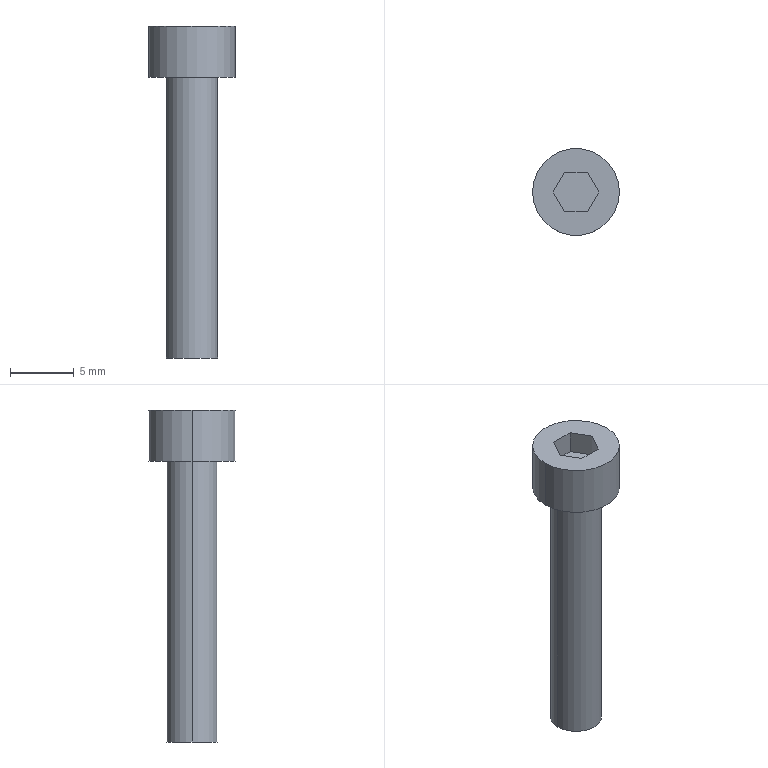Part | SolidWorks | features BaseBody 1 | 1 solid | 14 faces | box 6.8 x 6.8 x 26 mm | volume 406.575 mm3 | plane 10 | cylinder 4 | commonest cylinder face diameters 4 x2 6.8 x2
STEP:
#1=CARTESIAN_POINT('',(2.,0.,-22.));
#2=VERTEX_POINT('',#1);
#3=CARTESIAN_POINT('',(-2.,0.,-22.));
#4=VERTEX_POINT('',#3);
#5=CARTESIAN_POINT('',(0.,0.,-22.));
#6=DIRECTION('',(0.,0.,1.));
#7=DIRECTION('',(1.,0.,0.));
#8=AXIS2_PLACEMENT_3D('',#5,#6,#7);
#9=CIRCLE('',#8,2.);
#10=EDGE_CURVE('',#2,#4,#9,.T.);
#11=ORIENTED_EDGE('',*,*,#10,.T.);
#12=CARTESIAN_POINT('',(-2.,0.,0.));
#13=VERTEX_POINT('',#12);
#14=CARTESIAN_POINT('',(-2.,0.,-22.));
#15=DIRECTION('',(0.,0.,1.));
#16=VECTOR('',#15,1000.);
#17=LINE('',#14,#16);
#18=EDGE_CURVE('',#4,#13,#17,.T.);
#19=ORIENTED_EDGE('',*,*,#18,.T.);
#20=CARTESIAN_POINT('',(2.,0.,0.));
#21=VERTEX_POINT('',#20);
#22=CARTESIAN_POINT('',(0.,0.,0.));
#23=DIRECTION('',(0.,0.,-1.));
#24=DIRECTION('',(1.,0.,0.));
#25=AXIS2_PLACEMENT_3D('',#22,#23,#24);
#26=CIRCLE('',#25,2.);
#27=EDGE_CURVE('',#13,#21,#26,.T.);
#28=ORIENTED_EDGE('',*,*,#27,.T.);
#29=CARTESIAN_POINT('',(2.,0.,-22.));
#30=DIRECTION('',(0.,0.,1.));
#31=VECTOR('',#30,1000.);
#32=LINE('',#29,#31);
#33=EDGE_CURVE('',#2,#21,#32,.T.);
#34=ORIENTED_EDGE('',*,*,#33,.F.);
#35=EDGE_LOOP('',(#11,#19,#28,#34));
#36=FACE_OUTER_BOUND('',#35,.T.);
#37=CARTESIAN_POINT('',(0.,0.,-22.));
#38=DIRECTION('',(0.,0.,1.));
#39=DIRECTION('',(1.,0.,0.));
#40=AXIS2_PLACEMENT_3D('',#37,#38,#39);
#41=CYLINDRICAL_SURFACE('',#40,2.);
#42=ADVANCED_FACE('',(#36),#41,.T.);
#43=CARTESIAN_POINT('',(3.4,0.,0.));
#44=VERTEX_POINT('',#43);
#45=CARTESIAN_POINT('',(-3.4,0.,0.));
#46=VERTEX_POINT('',#45);
#47=CARTESIAN_POINT('',(0.,0.,0.));
#48=DIRECTION('',(0.,0.,1.));
#49=DIRECTION('',(1.,0.,0.));
#50=AXIS2_PLACEMENT_3D('',#47,#48,#49);
#51=CIRCLE('',#50,3.4);
#52=EDGE_CURVE('',#44,#46,#51,.T.);
#53=ORIENTED_EDGE('',*,*,#52,.T.);
#54=CARTESIAN_POINT('',(-3.4,0.,4.));
#55=VERTEX_POINT('',#54);
#56=CARTESIAN_POINT('',(-3.4,0.,0.));
#57=DIRECTION('',(0.,0.,1.));
#58=VECTOR('',#57,1000.);
#59=LINE('',#56,#58);
#60=EDGE_CURVE('',#46,#55,#59,.T.);
#61=ORIENTED_EDGE('',*,*,#60,.T.);
#62=CARTESIAN_POINT('',(3.4,0.,4.));
#63=VERTEX_POINT('',#62);
#64=CARTESIAN_POINT('',(0.,0.,4.));
#65=DIRECTION('',(0.,0.,-1.));
#66=DIRECTION('',(1.,0.,0.));
#67=AXIS2_PLACEMENT_3D('',#64,#65,#66);
#68=CIRCLE('',#67,3.4);
#69=EDGE_CURVE('',#55,#63,#68,.T.);
#70=ORIENTED_EDGE('',*,*,#69,.T.);
#71=CARTESIAN_POINT('',(3.4,0.,0.));
#72=DIRECTION('',(0.,0.,1.));
#73=VECTOR('',#72,1000.);
#74=LINE('',#71,#73);
#75=EDGE_CURVE('',#44,#63,#74,.T.);
#76=ORIENTED_EDGE('',*,*,#75,.F.);
#77=EDGE_LOOP('',(#53,#61,#70,#76));
#78=FACE_OUTER_BOUND('',#77,.T.);
#79=CARTESIAN_POINT('',(0.,0.,0.));
#80=DIRECTION('',(0.,0.,1.));
#81=DIRECTION('',(1.,0.,0.));
#82=AXIS2_PLACEMENT_3D('',#79,#80,#81);
#83=CYLINDRICAL_SURFACE('',#82,3.4);
#84=ADVANCED_FACE('',(#78),#83,.T.);
#85=ORIENTED_EDGE('',*,*,#18,.F.);
#86=CARTESIAN_POINT('',(0.,0.,-22.));
#87=DIRECTION('',(0.,0.,1.));
#88=DIRECTION('',(1.,0.,0.));
#89=AXIS2_PLACEMENT_3D('',#86,#87,#88);
#90=CIRCLE('',#89,2.);
#91=EDGE_CURVE('',#4,#2,#90,.T.);
#92=ORIENTED_EDGE('',*,*,#91,.T.);
#93=ORIENTED_EDGE('',*,*,#33,.T.);
#94=CARTESIAN_POINT('',(0.,0.,0.));
#95=DIRECTION('',(0.,0.,-1.));
#96=DIRECTION('',(1.,0.,0.));
#97=AXIS2_PLACEMENT_3D('',#94,#95,#96);
#98=CIRCLE('',#97,2.);
#99=EDGE_CURVE('',#21,#13,#98,.T.);
#100=ORIENTED_EDGE('',*,*,#99,.T.);
#101=EDGE_LOOP('',(#85,#92,#93,#100));
#102=FACE_OUTER_BOUND('',#101,.T.);
#103=CARTESIAN_POINT('',(0.,0.,-22.));
#104=DIRECTION('',(0.,0.,1.));
#105=DIRECTION('',(1.,0.,0.));
#106=AXIS2_PLACEMENT_3D('',#103,#104,#105);
#107=CYLINDRICAL_SURFACE('',#106,2.);
#108=ADVANCED_FACE('',(#102),#107,.T.);
#109=ORIENTED_EDGE('',*,*,#10,.F.);
#110=ORIENTED_EDGE('',*,*,#91,.F.);
#111=EDGE_LOOP('',(#109,#110));
#112=FACE_OUTER_BOUND('',#111,.T.);
#113=CARTESIAN_POINT('',(0.,0.,-22.));
#114=DIRECTION('',(0.,0.,1.));
#115=DIRECTION('',(1.,0.,0.));
#116=AXIS2_PLACEMENT_3D('',#113,#114,#115);
#117=PLANE('',#116);
#118=ADVANCED_FACE('',(#112),#117,.F.);
#119=ORIENTED_EDGE('',*,*,#99,.F.);
#120=ORIENTED_EDGE('',*,*,#27,.F.);
#121=EDGE_LOOP('',(#119,#120));
#122=FACE_BOUND('',#121,.T.);
#123=ORIENTED_EDGE('',*,*,#52,.F.);
#124=CARTESIAN_POINT('',(0.,0.,0.));
#125=DIRECTION('',(0.,0.,1.));
#126=DIRECTION('',(1.,0.,0.));
#127=AXIS2_PLACEMENT_3D('',#124,#125,#126);
#128=CIRCLE('',#127,3.4);
#129=EDGE_CURVE('',#46,#44,#128,.T.);
#130=ORIENTED_EDGE('',*,*,#129,.F.);
#131=EDGE_LOOP('',(#123,#130));
#132=FACE_OUTER_BOUND('',#131,.T.);
#133=CARTESIAN_POINT('',(0.,0.,0.));
#134=DIRECTION('',(0.,0.,1.));
#135=DIRECTION('',(1.,0.,0.));
#136=AXIS2_PLACEMENT_3D('',#133,#134,#135);
#137=PLANE('',#136);
#138=ADVANCED_FACE('',(#122,#132),#137,.F.);
#139=ORIENTED_EDGE('',*,*,#60,.F.);
#140=ORIENTED_EDGE('',*,*,#129,.T.);
#141=ORIENTED_EDGE('',*,*,#75,.T.);
#142=CARTESIAN_POINT('',(0.,0.,4.));
#143=DIRECTION('',(0.,0.,-1.));
#144=DIRECTION('',(1.,0.,0.));
#145=AXIS2_PLACEMENT_3D('',#142,#143,#144);
#146=CIRCLE('',#145,3.4);
#147=EDGE_CURVE('',#63,#55,#146,.T.);
#148=ORIENTED_EDGE('',*,*,#147,.T.);
#149=EDGE_LOOP('',(#139,#140,#141,#148));
#150=FACE_OUTER_BOUND('',#149,.T.);
#151=CARTESIAN_POINT('',(0.,0.,0.));
#152=DIRECTION('',(0.,0.,1.));
#153=DIRECTION('',(1.,0.,0.));
#154=AXIS2_PLACEMENT_3D('',#151,#152,#153);
#155=CYLINDRICAL_SURFACE('',#154,3.4);
#156=ADVANCED_FACE('',(#150),#155,.T.);
#157=CARTESIAN_POINT('',(-0.9,-1.559,4.));
#158=VERTEX_POINT('',#157);
#159=CARTESIAN_POINT('',(-1.8,0.,4.));
#160=VERTEX_POINT('',#159);
#161=CARTESIAN_POINT('',(-0.9,-1.559,4.));
#162=DIRECTION('',(-0.5,0.866,0.));
#163=VECTOR('',#162,1000.);
#164=LINE('',#161,#163);
#165=EDGE_CURVE('',#158,#160,#164,.T.);
#166=ORIENTED_EDGE('',*,*,#165,.T.);
#167=CARTESIAN_POINT('',(-0.9,1.559,4.));
#168=VERTEX_POINT('',#167);
#169=CARTESIAN_POINT('',(-1.8,0.,4.));
#170=DIRECTION('',(0.5,0.866,0.));
#171=VECTOR('',#170,1000.);
#172=LINE('',#169,#171);
#173=EDGE_CURVE('',#160,#168,#172,.T.);
#174=ORIENTED_EDGE('',*,*,#173,.T.);
#175=CARTESIAN_POINT('',(0.9,1.559,4.));
#176=VERTEX_POINT('',#175);
#177=CARTESIAN_POINT('',(0.,1.559,4.));
#178=DIRECTION('',(1.,0.,0.));
#179=VECTOR('',#178,1000.);
#180=LINE('',#177,#179);
#181=EDGE_CURVE('',#168,#176,#180,.T.);
#182=ORIENTED_EDGE('',*,*,#181,.T.);
#183=CARTESIAN_POINT('',(1.8,0.,4.));
#184=VERTEX_POINT('',#183);
#185=CARTESIAN_POINT('',(0.9,1.559,4.));
#186=DIRECTION('',(0.5,-0.866,0.));
#187=VECTOR('',#186,1000.);
#188=LINE('',#185,#187);
#189=EDGE_CURVE('',#176,#184,#188,.T.);
#190=ORIENTED_EDGE('',*,*,#189,.T.);
#191=CARTESIAN_POINT('',(0.9,-1.559,4.));
#192=VERTEX_POINT('',#191);
#193=CARTESIAN_POINT('',(1.8,0.,4.));
#194=DIRECTION('',(-0.5,-0.866,0.));
#195=VECTOR('',#194,1000.);
#196=LINE('',#193,#195);
#197=EDGE_CURVE('',#184,#192,#196,.T.);
#198=ORIENTED_EDGE('',*,*,#197,.T.);
#199=CARTESIAN_POINT('',(0.,-1.559,4.));
#200=DIRECTION('',(-1.,0.,0.));
#201=VECTOR('',#200,1000.);
#202=LINE('',#199,#201);
#203=EDGE_CURVE('',#192,#158,#202,.T.);
#204=ORIENTED_EDGE('',*,*,#203,.T.);
#205=EDGE_LOOP('',(#166,#174,#182,#190,#198,#204));
#206=FACE_BOUND('',#205,.T.);
#207=ORIENTED_EDGE('',*,*,#147,.F.);
#208=ORIENTED_EDGE('',*,*,#69,.F.);
#209=EDGE_LOOP('',(#207,#208));
#210=FACE_OUTER_BOUND('',#209,.T.);
#211=CARTESIAN_POINT('',(0.,0.,4.));
#212=DIRECTION('',(0.,0.,1.));
#213=DIRECTION('',(1.,0.,0.));
#214=AXIS2_PLACEMENT_3D('',#211,#212,#213);
#215=PLANE('',#214);
#216=ADVANCED_FACE('',(#206,#210),#215,.T.);
#217=ORIENTED_EDGE('',*,*,#173,.F.);
#218=CARTESIAN_POINT('',(-1.8,0.,2.2));
#219=VERTEX_POINT('',#218);
#220=CARTESIAN_POINT('',(-1.8,0.,2.2));
#221=DIRECTION('',(0.,0.,-1.));
#222=VECTOR('',#221,1000.);
#223=LINE('',#220,#222);
#224=EDGE_CURVE('',#160,#219,#223,.T.);
#225=ORIENTED_EDGE('',*,*,#224,.T.);
#226=CARTESIAN_POINT('',(-0.9,1.559,2.2));
#227=VERTEX_POINT('',#226);
#228=CARTESIAN_POINT('',(-0.9,1.559,2.2));
#229=DIRECTION('',(0.5,0.866,0.));
#230=VECTOR('',#229,1000.);
#231=LINE('',#228,#230);
#232=EDGE_CURVE('',#219,#227,#231,.T.);
#233=ORIENTED_EDGE('',*,*,#232,.T.);
#234=CARTESIAN_POINT('',(-0.9,1.559,2.2));
#235=DIRECTION('',(0.,0.,1.));
#236=VECTOR('',#235,1000.);
#237=LINE('',#234,#236);
#238=EDGE_CURVE('',#227,#168,#237,.T.);
#239=ORIENTED_EDGE('',*,*,#238,.T.);
#240=EDGE_LOOP('',(#217,#225,#233,#239));
#241=FACE_OUTER_BOUND('',#240,.T.);
#242=CARTESIAN_POINT('',(-0.9,1.559,2.2));
#243=DIRECTION('',(0.866,-0.5,0.));
#244=DIRECTION('',(0.5,0.866,0.));
#245=AXIS2_PLACEMENT_3D('',#242,#243,#244);
#246=PLANE('',#245);
#247=ADVANCED_FACE('',(#241),#246,.T.);
#248=ORIENTED_EDGE('',*,*,#165,.F.);
#249=CARTESIAN_POINT('',(-0.9,-1.559,2.2));
#250=VERTEX_POINT('',#249);
#251=CARTESIAN_POINT('',(-0.9,-1.559,2.2));
#252=DIRECTION('',(0.,0.,-1.));
#253=VECTOR('',#252,1000.);
#254=LINE('',#251,#253);
#255=EDGE_CURVE('',#158,#250,#254,.T.);
#256=ORIENTED_EDGE('',*,*,#255,.T.);
#257=CARTESIAN_POINT('',(-1.8,0.,2.2));
#258=DIRECTION('',(-0.5,0.866,0.));
#259=VECTOR('',#258,1000.);
#260=LINE('',#257,#259);
#261=EDGE_CURVE('',#250,#219,#260,.T.);
#262=ORIENTED_EDGE('',*,*,#261,.T.);
#263=ORIENTED_EDGE('',*,*,#224,.F.);
#264=EDGE_LOOP('',(#248,#256,#262,#263));
#265=FACE_OUTER_BOUND('',#264,.T.);
#266=CARTESIAN_POINT('',(-1.8,0.,2.2));
#267=DIRECTION('',(0.866,0.5,0.));
#268=DIRECTION('',(-0.5,0.866,0.));
#269=AXIS2_PLACEMENT_3D('',#266,#267,#268);
#270=PLANE('',#269);
#271=ADVANCED_FACE('',(#265),#270,.T.);
#272=ORIENTED_EDGE('',*,*,#203,.F.);
#273=CARTESIAN_POINT('',(0.9,-1.559,2.2));
#274=VERTEX_POINT('',#273);
#275=CARTESIAN_POINT('',(0.9,-1.559,2.2));
#276=DIRECTION('',(0.,0.,-1.));
#277=VECTOR('',#276,1000.);
#278=LINE('',#275,#277);
#279=EDGE_CURVE('',#192,#274,#278,.T.);
#280=ORIENTED_EDGE('',*,*,#279,.T.);
#281=CARTESIAN_POINT('',(-0.9,-1.559,2.2));
#282=DIRECTION('',(-1.,0.,0.));
#283=VECTOR('',#282,1000.);
#284=LINE('',#281,#283);
#285=EDGE_CURVE('',#274,#250,#284,.T.);
#286=ORIENTED_EDGE('',*,*,#285,.T.);
#287=ORIENTED_EDGE('',*,*,#255,.F.);
#288=EDGE_LOOP('',(#272,#280,#286,#287));
#289=FACE_OUTER_BOUND('',#288,.T.);
#290=CARTESIAN_POINT('',(-0.9,-1.559,2.2));
#291=DIRECTION('',(0.,1.,0.));
#292=DIRECTION('',(-1.,0.,0.));
#293=AXIS2_PLACEMENT_3D('',#290,#291,#292);
#294=PLANE('',#293);
#295=ADVANCED_FACE('',(#289),#294,.T.);
#296=ORIENTED_EDGE('',*,*,#197,.F.);
#297=CARTESIAN_POINT('',(1.8,0.,2.2));
#298=VERTEX_POINT('',#297);
#299=CARTESIAN_POINT('',(1.8,0.,2.2));
#300=DIRECTION('',(0.,0.,-1.));
#301=VECTOR('',#300,1000.);
#302=LINE('',#299,#301);
#303=EDGE_CURVE('',#184,#298,#302,.T.);
#304=ORIENTED_EDGE('',*,*,#303,.T.);
#305=CARTESIAN_POINT('',(0.9,-1.559,2.2));
#306=DIRECTION('',(-0.5,-0.866,0.));
#307=VECTOR('',#306,1000.);
#308=LINE('',#305,#307);
#309=EDGE_CURVE('',#298,#274,#308,.T.);
#310=ORIENTED_EDGE('',*,*,#309,.T.);
#311=ORIENTED_EDGE('',*,*,#279,.F.);
#312=EDGE_LOOP('',(#296,#304,#310,#311));
#313=FACE_OUTER_BOUND('',#312,.T.);
#314=CARTESIAN_POINT('',(0.9,-1.559,2.2));
#315=DIRECTION('',(-0.866,0.5,0.));
#316=DIRECTION('',(-0.5,-0.866,0.));
#317=AXIS2_PLACEMENT_3D('',#314,#315,#316);
#318=PLANE('',#317);
#319=ADVANCED_FACE('',(#313),#318,.T.);
#320=ORIENTED_EDGE('',*,*,#189,.F.);
#321=CARTESIAN_POINT('',(0.9,1.559,2.2));
#322=VERTEX_POINT('',#321);
#323=CARTESIAN_POINT('',(0.9,1.559,2.2));
#324=DIRECTION('',(0.,0.,-1.));
#325=VECTOR('',#324,1000.);
#326=LINE('',#323,#325);
#327=EDGE_CURVE('',#176,#322,#326,.T.);
#328=ORIENTED_EDGE('',*,*,#327,.T.);
#329=CARTESIAN_POINT('',(1.8,0.,2.2));
#330=DIRECTION('',(0.5,-0.866,0.));
#331=VECTOR('',#330,1000.);
#332=LINE('',#329,#331);
#333=EDGE_CURVE('',#322,#298,#332,.T.);
#334=ORIENTED_EDGE('',*,*,#333,.T.);
#335=ORIENTED_EDGE('',*,*,#303,.F.);
#336=EDGE_LOOP('',(#320,#328,#334,#335));
#337=FACE_OUTER_BOUND('',#336,.T.);
#338=CARTESIAN_POINT('',(1.8,0.,2.2));
#339=DIRECTION('',(-0.866,-0.5,0.));
#340=DIRECTION('',(0.5,-0.866,0.));
#341=AXIS2_PLACEMENT_3D('',#338,#339,#340);
#342=PLANE('',#341);
#343=ADVANCED_FACE('',(#337),#342,.T.);
#344=ORIENTED_EDGE('',*,*,#181,.F.);
#345=ORIENTED_EDGE('',*,*,#238,.F.);
#346=CARTESIAN_POINT('',(0.9,1.559,2.2));
#347=DIRECTION('',(1.,0.,0.));
#348=VECTOR('',#347,1000.);
#349=LINE('',#346,#348);
#350=EDGE_CURVE('',#227,#322,#349,.T.);
#351=ORIENTED_EDGE('',*,*,#350,.T.);
#352=ORIENTED_EDGE('',*,*,#327,.F.);
#353=EDGE_LOOP('',(#344,#345,#351,#352));
#354=FACE_OUTER_BOUND('',#353,.T.);
#355=CARTESIAN_POINT('',(0.9,1.559,2.2));
#356=DIRECTION('',(0.,-1.,0.));
#357=DIRECTION('',(1.,0.,0.));
#358=AXIS2_PLACEMENT_3D('',#355,#356,#357);
#359=PLANE('',#358);
#360=ADVANCED_FACE('',(#354),#359,.T.);
#361=ORIENTED_EDGE('',*,*,#285,.F.);
#362=ORIENTED_EDGE('',*,*,#309,.F.);
#363=ORIENTED_EDGE('',*,*,#333,.F.);
#364=ORIENTED_EDGE('',*,*,#350,.F.);
#365=ORIENTED_EDGE('',*,*,#232,.F.);
#366=ORIENTED_EDGE('',*,*,#261,.F.);
#367=EDGE_LOOP('',(#361,#362,#363,#364,#365,#366));
#368=FACE_OUTER_BOUND('',#367,.T.);
#369=CARTESIAN_POINT('',(0.,0.,2.2));
#370=DIRECTION('',(0.,0.,1.));
#371=DIRECTION('',(1.,0.,0.));
#372=AXIS2_PLACEMENT_3D('',#369,#370,#371);
#373=PLANE('',#372);
#374=ADVANCED_FACE('',(#368),#373,.T.);
#375=CLOSED_SHELL('',(#42,#84,#108,#118,#138,#156,#216,#247,#271,#295,#319,#343,#360,#374));
#376=MANIFOLD_SOLID_BREP('',#375);
#377=CARTESIAN_POINT('',(0.,0.,0.));
#378=DIRECTION('',(0.,0.,1.));
#379=DIRECTION('',(1.,0.,0.));
#380=AXIS2_PLACEMENT_3D('',#377,#378,#379);
#381=(LENGTH_UNIT()NAMED_UNIT(*)SI_UNIT(.MILLI.,.METRE.));
#382=UNCERTAINTY_MEASURE_WITH_UNIT(LENGTH_MEASURE(0.00001),#381,'','');
#383=(NAMED_UNIT(*)PLANE_ANGLE_UNIT()SI_UNIT($,.RADIAN.));
#384=(NAMED_UNIT(*)SI_UNIT($,.STERADIAN.)SOLID_ANGLE_UNIT());
#385=(GEOMETRIC_REPRESENTATION_CONTEXT(3)GLOBAL_UNCERTAINTY_ASSIGNED_CONTEXT((#382))GLOBAL_UNIT_ASSIGNED_CONTEXT((#381,#383,#384))REPRESENTATION_CONTEXT('',''));
#386=ADVANCED_BREP_SHAPE_REPRESENTATION('',(#376,#380),#385);